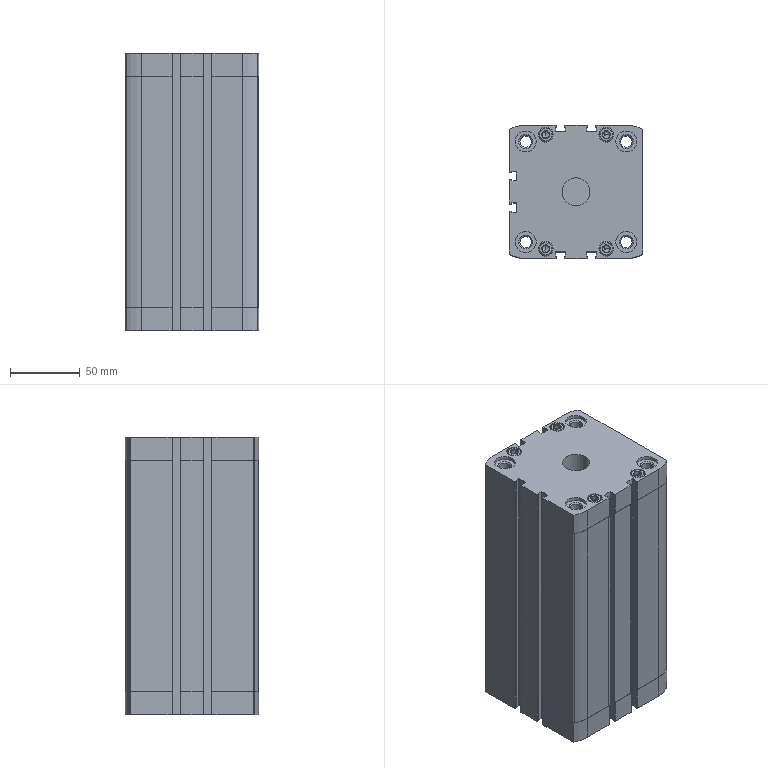Part | SolidWorks | features BaseBody 1 | 1 solid | 465 faces | box 95.5 x 95.5 x 199 mm | volume 863513 mm3 | plane 219 | cylinder 178 | cone 68 | commonest cylinder face diameters 0.8 x48 0.4 x24 8.376 x16 10 x16 10.7 x16 15 x16